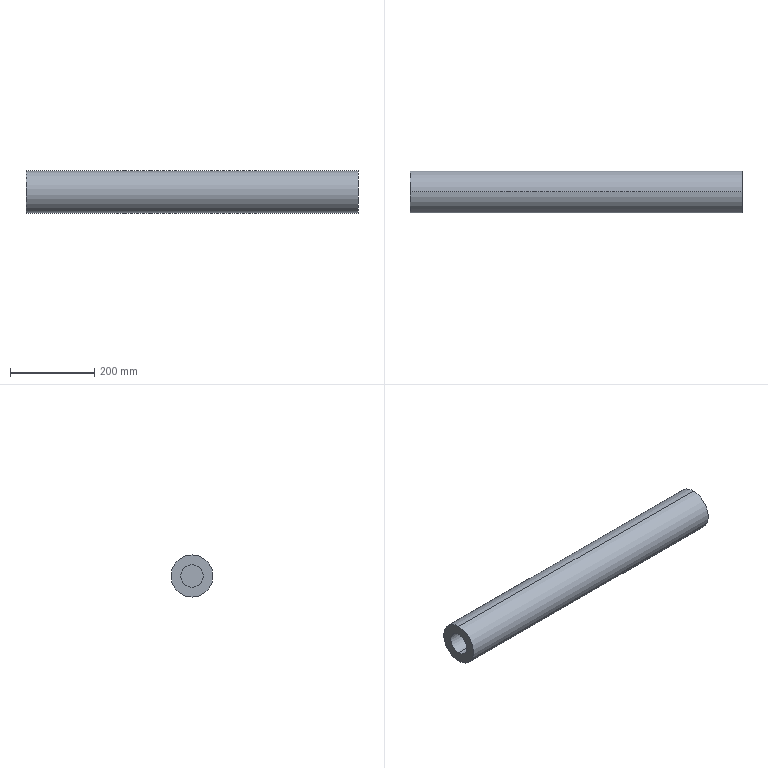Part | SolidWorks | 1 solid | 10 faces | box 787.42 x 100 x 100 mm | volume 5924053 mm3 | cylinder 6 | plane 4 | commonest cylinder face diameters 53 x4 100 x2
STEP:
#1=CARTESIAN_POINT('',(718.42,0.,-26.5));
#2=VERTEX_POINT('',#1);
#3=CARTESIAN_POINT('',(718.42,0.,26.5));
#4=VERTEX_POINT('',#3);
#5=CARTESIAN_POINT('',(718.42,0.,0.));
#6=DIRECTION('',(-1.,0.,0.));
#7=DIRECTION('',(0.,0.,-1.));
#8=AXIS2_PLACEMENT_3D('',#5,#6,#7);
#9=CIRCLE('',#8,26.5);
#10=EDGE_CURVE('',#2,#4,#9,.T.);
#11=ORIENTED_EDGE('',*,*,#10,.T.);
#12=CARTESIAN_POINT('',(787.42,0.,26.5));
#13=VERTEX_POINT('',#12);
#14=CARTESIAN_POINT('',(718.42,0.,26.5));
#15=DIRECTION('',(1.,0.,0.));
#16=VECTOR('',#15,1000.);
#17=LINE('',#14,#16);
#18=EDGE_CURVE('',#4,#13,#17,.T.);
#19=ORIENTED_EDGE('',*,*,#18,.T.);
#20=CARTESIAN_POINT('',(787.42,0.,-26.5));
#21=VERTEX_POINT('',#20);
#22=CARTESIAN_POINT('',(787.42,0.,0.));
#23=DIRECTION('',(1.,0.,0.));
#24=DIRECTION('',(0.,0.,1.));
#25=AXIS2_PLACEMENT_3D('',#22,#23,#24);
#26=CIRCLE('',#25,26.5);
#27=EDGE_CURVE('',#13,#21,#26,.T.);
#28=ORIENTED_EDGE('',*,*,#27,.T.);
#29=CARTESIAN_POINT('',(718.42,0.,-26.5));
#30=DIRECTION('',(1.,0.,0.));
#31=VECTOR('',#30,1000.);
#32=LINE('',#29,#31);
#33=EDGE_CURVE('',#2,#21,#32,.T.);
#34=ORIENTED_EDGE('',*,*,#33,.F.);
#35=EDGE_LOOP('',(#11,#19,#28,#34));
#36=FACE_OUTER_BOUND('',#35,.T.);
#37=CARTESIAN_POINT('',(787.42,0.,0.));
#38=DIRECTION('',(-1.,0.,0.));
#39=DIRECTION('',(0.,0.,1.));
#40=AXIS2_PLACEMENT_3D('',#37,#38,#39);
#41=CYLINDRICAL_SURFACE('',#40,26.5);
#42=ADVANCED_FACE('',(#36),#41,.F.);
#43=CARTESIAN_POINT('',(49.,0.,-26.5));
#44=VERTEX_POINT('',#43);
#45=CARTESIAN_POINT('',(49.,0.,26.5));
#46=VERTEX_POINT('',#45);
#47=CARTESIAN_POINT('',(49.,0.,0.));
#48=DIRECTION('',(1.,0.,0.));
#49=DIRECTION('',(0.,0.,-1.));
#50=AXIS2_PLACEMENT_3D('',#47,#48,#49);
#51=CIRCLE('',#50,26.5);
#52=EDGE_CURVE('',#44,#46,#51,.T.);
#53=ORIENTED_EDGE('',*,*,#52,.F.);
#54=CARTESIAN_POINT('',(49.,0.,0.));
#55=DIRECTION('',(1.,0.,0.));
#56=DIRECTION('',(0.,0.,1.));
#57=AXIS2_PLACEMENT_3D('',#54,#55,#56);
#58=CIRCLE('',#57,26.5);
#59=EDGE_CURVE('',#46,#44,#58,.T.);
#60=ORIENTED_EDGE('',*,*,#59,.F.);
#61=EDGE_LOOP('',(#53,#60));
#62=FACE_OUTER_BOUND('',#61,.T.);
#63=CARTESIAN_POINT('',(49.,0.,0.));
#64=DIRECTION('',(1.,0.,0.));
#65=DIRECTION('',(0.,1.,0.));
#66=AXIS2_PLACEMENT_3D('',#63,#64,#65);
#67=PLANE('',#66);
#68=ADVANCED_FACE('',(#62),#67,.F.);
#69=CARTESIAN_POINT('',(0.,0.,26.5));
#70=VERTEX_POINT('',#69);
#71=CARTESIAN_POINT('',(0.,0.,26.5));
#72=DIRECTION('',(1.,0.,0.));
#73=VECTOR('',#72,1000.);
#74=LINE('',#71,#73);
#75=EDGE_CURVE('',#70,#46,#74,.T.);
#76=ORIENTED_EDGE('',*,*,#75,.F.);
#77=CARTESIAN_POINT('',(0.,0.,-26.5));
#78=VERTEX_POINT('',#77);
#79=CARTESIAN_POINT('',(0.,0.,0.));
#80=DIRECTION('',(-1.,0.,0.));
#81=DIRECTION('',(0.,0.,1.));
#82=AXIS2_PLACEMENT_3D('',#79,#80,#81);
#83=CIRCLE('',#82,26.5);
#84=EDGE_CURVE('',#70,#78,#83,.T.);
#85=ORIENTED_EDGE('',*,*,#84,.T.);
#86=CARTESIAN_POINT('',(0.,0.,-26.5));
#87=DIRECTION('',(1.,0.,0.));
#88=VECTOR('',#87,1000.);
#89=LINE('',#86,#88);
#90=EDGE_CURVE('',#78,#44,#89,.T.);
#91=ORIENTED_EDGE('',*,*,#90,.T.);
#92=ORIENTED_EDGE('',*,*,#52,.T.);
#93=EDGE_LOOP('',(#76,#85,#91,#92));
#94=FACE_OUTER_BOUND('',#93,.T.);
#95=CARTESIAN_POINT('',(49.,0.,0.));
#96=DIRECTION('',(-1.,0.,0.));
#97=DIRECTION('',(0.,0.,1.));
#98=AXIS2_PLACEMENT_3D('',#95,#96,#97);
#99=CYLINDRICAL_SURFACE('',#98,26.5);
#100=ADVANCED_FACE('',(#94),#99,.F.);
#101=CARTESIAN_POINT('',(0.,0.,0.));
#102=DIRECTION('',(-1.,0.,0.));
#103=DIRECTION('',(0.,0.,-1.));
#104=AXIS2_PLACEMENT_3D('',#101,#102,#103);
#105=CIRCLE('',#104,26.5);
#106=EDGE_CURVE('',#78,#70,#105,.T.);
#107=ORIENTED_EDGE('',*,*,#106,.T.);
#108=ORIENTED_EDGE('',*,*,#75,.T.);
#109=ORIENTED_EDGE('',*,*,#59,.T.);
#110=ORIENTED_EDGE('',*,*,#90,.F.);
#111=EDGE_LOOP('',(#107,#108,#109,#110));
#112=FACE_OUTER_BOUND('',#111,.T.);
#113=CARTESIAN_POINT('',(49.,0.,0.));
#114=DIRECTION('',(-1.,0.,0.));
#115=DIRECTION('',(0.,0.,1.));
#116=AXIS2_PLACEMENT_3D('',#113,#114,#115);
#117=CYLINDRICAL_SURFACE('',#116,26.5);
#118=ADVANCED_FACE('',(#112),#117,.F.);
#119=ORIENTED_EDGE('',*,*,#84,.F.);
#120=ORIENTED_EDGE('',*,*,#106,.F.);
#121=EDGE_LOOP('',(#119,#120));
#122=FACE_BOUND('',#121,.T.);
#123=CARTESIAN_POINT('',(0.,0.,50.));
#124=VERTEX_POINT('',#123);
#125=CARTESIAN_POINT('',(0.,0.,-50.));
#126=VERTEX_POINT('',#125);
#127=CARTESIAN_POINT('',(0.,0.,0.));
#128=DIRECTION('',(1.,0.,0.));
#129=DIRECTION('',(0.,0.,1.));
#130=AXIS2_PLACEMENT_3D('',#127,#128,#129);
#131=CIRCLE('',#130,50.);
#132=EDGE_CURVE('',#124,#126,#131,.T.);
#133=ORIENTED_EDGE('',*,*,#132,.F.);
#134=CARTESIAN_POINT('',(0.,0.,0.));
#135=DIRECTION('',(1.,0.,0.));
#136=DIRECTION('',(0.,0.,-1.));
#137=AXIS2_PLACEMENT_3D('',#134,#135,#136);
#138=CIRCLE('',#137,50.);
#139=EDGE_CURVE('',#126,#124,#138,.T.);
#140=ORIENTED_EDGE('',*,*,#139,.F.);
#141=EDGE_LOOP('',(#133,#140));
#142=FACE_OUTER_BOUND('',#141,.T.);
#143=CARTESIAN_POINT('',(0.,0.,0.));
#144=DIRECTION('',(1.,0.,0.));
#145=DIRECTION('',(0.,1.,0.));
#146=AXIS2_PLACEMENT_3D('',#143,#144,#145);
#147=PLANE('',#146);
#148=ADVANCED_FACE('',(#122,#142),#147,.F.);
#149=ORIENTED_EDGE('',*,*,#139,.T.);
#150=CARTESIAN_POINT('',(787.42,0.,50.));
#151=VERTEX_POINT('',#150);
#152=CARTESIAN_POINT('',(0.,0.,50.));
#153=DIRECTION('',(1.,0.,0.));
#154=VECTOR('',#153,1000.);
#155=LINE('',#152,#154);
#156=EDGE_CURVE('',#124,#151,#155,.T.);
#157=ORIENTED_EDGE('',*,*,#156,.T.);
#158=CARTESIAN_POINT('',(787.42,0.,-50.));
#159=VERTEX_POINT('',#158);
#160=CARTESIAN_POINT('',(787.42,0.,0.));
#161=DIRECTION('',(-1.,0.,0.));
#162=DIRECTION('',(0.,0.,1.));
#163=AXIS2_PLACEMENT_3D('',#160,#161,#162);
#164=CIRCLE('',#163,50.);
#165=EDGE_CURVE('',#151,#159,#164,.T.);
#166=ORIENTED_EDGE('',*,*,#165,.T.);
#167=CARTESIAN_POINT('',(0.,0.,-50.));
#168=DIRECTION('',(1.,0.,0.));
#169=VECTOR('',#168,1000.);
#170=LINE('',#167,#169);
#171=EDGE_CURVE('',#126,#159,#170,.T.);
#172=ORIENTED_EDGE('',*,*,#171,.F.);
#173=EDGE_LOOP('',(#149,#157,#166,#172));
#174=FACE_OUTER_BOUND('',#173,.T.);
#175=CARTESIAN_POINT('',(49.,0.,0.));
#176=DIRECTION('',(-1.,0.,0.));
#177=DIRECTION('',(0.,0.,1.));
#178=AXIS2_PLACEMENT_3D('',#175,#176,#177);
#179=CYLINDRICAL_SURFACE('',#178,50.);
#180=ADVANCED_FACE('',(#174),#179,.T.);
#181=ORIENTED_EDGE('',*,*,#156,.F.);
#182=ORIENTED_EDGE('',*,*,#132,.T.);
#183=ORIENTED_EDGE('',*,*,#171,.T.);
#184=CARTESIAN_POINT('',(787.42,0.,0.));
#185=DIRECTION('',(-1.,0.,0.));
#186=DIRECTION('',(0.,0.,-1.));
#187=AXIS2_PLACEMENT_3D('',#184,#185,#186);
#188=CIRCLE('',#187,50.);
#189=EDGE_CURVE('',#159,#151,#188,.T.);
#190=ORIENTED_EDGE('',*,*,#189,.T.);
#191=EDGE_LOOP('',(#181,#182,#183,#190));
#192=FACE_OUTER_BOUND('',#191,.T.);
#193=CARTESIAN_POINT('',(49.,0.,0.));
#194=DIRECTION('',(-1.,0.,0.));
#195=DIRECTION('',(0.,0.,1.));
#196=AXIS2_PLACEMENT_3D('',#193,#194,#195);
#197=CYLINDRICAL_SURFACE('',#196,50.);
#198=ADVANCED_FACE('',(#192),#197,.T.);
#199=CARTESIAN_POINT('',(787.42,0.,0.));
#200=DIRECTION('',(1.,0.,0.));
#201=DIRECTION('',(0.,0.,-1.));
#202=AXIS2_PLACEMENT_3D('',#199,#200,#201);
#203=CIRCLE('',#202,26.5);
#204=EDGE_CURVE('',#21,#13,#203,.T.);
#205=ORIENTED_EDGE('',*,*,#204,.F.);
#206=ORIENTED_EDGE('',*,*,#27,.F.);
#207=EDGE_LOOP('',(#205,#206));
#208=FACE_BOUND('',#207,.T.);
#209=ORIENTED_EDGE('',*,*,#165,.F.);
#210=ORIENTED_EDGE('',*,*,#189,.F.);
#211=EDGE_LOOP('',(#209,#210));
#212=FACE_OUTER_BOUND('',#211,.T.);
#213=CARTESIAN_POINT('',(787.42,0.,0.));
#214=DIRECTION('',(1.,0.,0.));
#215=DIRECTION('',(0.,1.,0.));
#216=AXIS2_PLACEMENT_3D('',#213,#214,#215);
#217=PLANE('',#216);
#218=ADVANCED_FACE('',(#208,#212),#217,.T.);
#219=ORIENTED_EDGE('',*,*,#18,.F.);
#220=CARTESIAN_POINT('',(718.42,0.,0.));
#221=DIRECTION('',(-1.,0.,0.));
#222=DIRECTION('',(0.,0.,1.));
#223=AXIS2_PLACEMENT_3D('',#220,#221,#222);
#224=CIRCLE('',#223,26.5);
#225=EDGE_CURVE('',#4,#2,#224,.T.);
#226=ORIENTED_EDGE('',*,*,#225,.T.);
#227=ORIENTED_EDGE('',*,*,#33,.T.);
#228=ORIENTED_EDGE('',*,*,#204,.T.);
#229=EDGE_LOOP('',(#219,#226,#227,#228));
#230=FACE_OUTER_BOUND('',#229,.T.);
#231=CARTESIAN_POINT('',(787.42,0.,0.));
#232=DIRECTION('',(-1.,0.,0.));
#233=DIRECTION('',(0.,0.,1.));
#234=AXIS2_PLACEMENT_3D('',#231,#232,#233);
#235=CYLINDRICAL_SURFACE('',#234,26.5);
#236=ADVANCED_FACE('',(#230),#235,.F.);
#237=ORIENTED_EDGE('',*,*,#10,.F.);
#238=ORIENTED_EDGE('',*,*,#225,.F.);
#239=EDGE_LOOP('',(#237,#238));
#240=FACE_OUTER_BOUND('',#239,.T.);
#241=CARTESIAN_POINT('',(718.42,0.,0.));
#242=DIRECTION('',(1.,0.,0.));
#243=DIRECTION('',(0.,1.,0.));
#244=AXIS2_PLACEMENT_3D('',#241,#242,#243);
#245=PLANE('',#244);
#246=ADVANCED_FACE('',(#240),#245,.T.);
#247=CLOSED_SHELL('',(#42,#68,#100,#118,#148,#180,#198,#218,#236,#246));
#248=MANIFOLD_SOLID_BREP('',#247);
#249=CARTESIAN_POINT('',(0.,0.,0.));
#250=DIRECTION('',(0.,0.,1.));
#251=DIRECTION('',(1.,0.,0.));
#252=AXIS2_PLACEMENT_3D('',#249,#250,#251);
#253=(LENGTH_UNIT()NAMED_UNIT(*)SI_UNIT(.MILLI.,.METRE.));
#254=UNCERTAINTY_MEASURE_WITH_UNIT(LENGTH_MEASURE(0.00001),#253,'','');
#255=(NAMED_UNIT(*)PLANE_ANGLE_UNIT()SI_UNIT($,.RADIAN.));
#256=(NAMED_UNIT(*)SI_UNIT($,.STERADIAN.)SOLID_ANGLE_UNIT());
#257=(GEOMETRIC_REPRESENTATION_CONTEXT(3)GLOBAL_UNCERTAINTY_ASSIGNED_CONTEXT((#254))GLOBAL_UNIT_ASSIGNED_CONTEXT((#253,#255,#256))REPRESENTATION_CONTEXT('',''));
#258=ADVANCED_BREP_SHAPE_REPRESENTATION('',(#248,#252),#257);